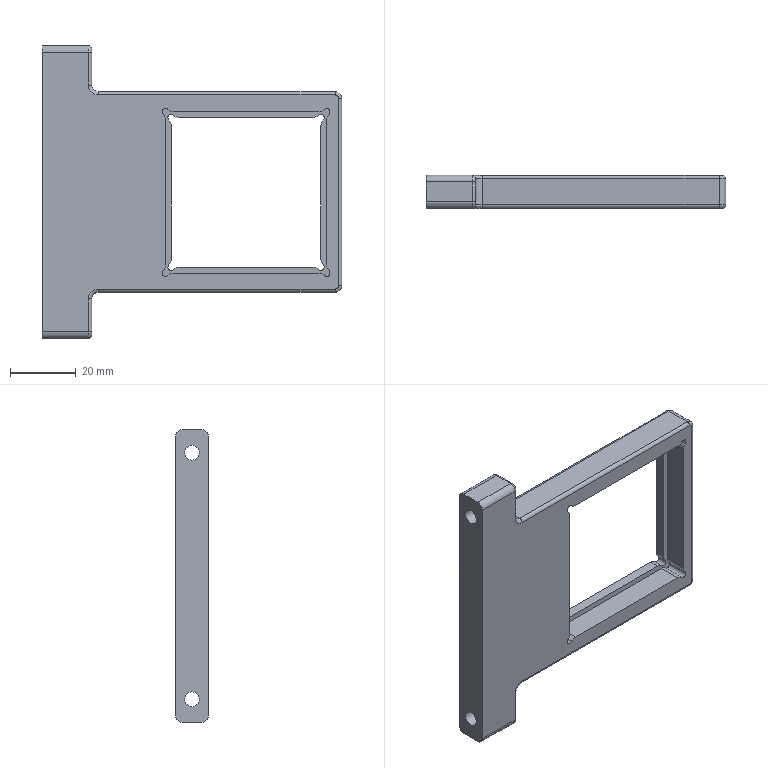NC program | NX | posted by the shop | part box 91 x 10 x 89 mm
Lines 39 to 1092 of 16928:
N2 T09 M06
(D10  D=10. R=0. H=09 ce=0.10 di=0.10)
G00 G90 G54 X33.301 Y3.249 M03 S8000
G43 H09 Z10.2
M08
Z1.5
G02 X33.301 Y3.249 Z1.006 I-2.966 J-3.384 F3000.
X33.301 Y3.249 Z.513 I-2.966 J-3.384
X33.301 Y3.249 Z.019 I-2.966 J-3.384
X33.301 Y3.249 Z-.474 I-2.966 J-3.384
X34.017 Y2.453 Z-.493 I-2.966 J-3.384
G01 X35.835 Y-.135
Y-19.535
X-2.965
Y19.265
X35.835
Y-2.121
G02 X35.417 Y-2.934 I-1. J0.0
G01 X29.254 Y-7.336
G03 X28.835 Y-8.149 I.581 J-.814
G01 Y-11.536
G02 X27.836 Y-12.535 I-1. J.001
G01 X5.034
G02 X4.035 Y-11.536 I.001 J1.
G01 Y11.266
G02 X5.034 Y12.265 I1. J-.001
G01 X27.836
G02 X28.835 Y11.266 I-.001 J-1.
G01 Y-1.878
G02 X28.107 Y-2.84 I-1. J0.0
G01 X22.354 Y-4.462
G03 X21.731 Y-4.98 I.272 J-.962
G02 X20.836 Y-5.535 I-.896 J.445
G01 X12.034
G02 X11.035 Y-4.536 I.001 J1.
G01 Y4.266
G02 X12.034 Y5.265 I1. J-.001
G01 X20.836
G02 X21.835 Y4.266 I-.001 J-1.
G01 X21.833 Y-1.135
G02 X21.033 Y-1.935 I-.8 J0.0
G01 X20.877 Y-1.919
X16.63 Y-1.074
G03 X16.34 Y-1.03 I-.631 J-3.173
G02 X15.535 Y-.135 I.095 J.895
X16.435 Y.765 I.9 J0.0
X17.335 Y-.135 I0.0 J-.9
X17.128 Y-.709 I-.9 J0.0
X16.721 Y-.988 I-.693 J.574
G03 X11.943 Y-7.626 I2.222 J-6.638
X12.305 Y-9.848 I7. J0.0
G01 Z.707
G00 Z3.
G01 X33.301 Y3.249 F6000.
G00 Z1.007
G02 X33.301 Y3.249 Z.514 I-2.966 J-3.384 F3000.
X33.301 Y3.249 Z.02 I-2.966 J-3.384
X33.301 Y3.249 Z-.473 I-2.966 J-3.384
X33.301 Y3.249 Z-.967 I-2.966 J-3.384
X34.017 Y2.453 Z-.986 I-2.966 J-3.384
G01 X35.835 Y-.135
Y-19.535
X-2.965
Y19.265
X35.835
Y-5.135
G02 X35.073 Y-6.106 I-1. J0.0
G01 X29.597 Y-7.448
G03 X28.835 Y-8.419 I.238 J-.971
G01 Y-11.536
G02 X27.836 Y-12.535 I-1. J.001
G01 X5.034
G02 X4.035 Y-11.536 I.001 J1.
G01 Y11.266
G02 X5.034 Y12.265 I1. J-.001
G01 X27.836
G02 X28.835 Y11.266 I-.001 J-1.
G01 Y-1.878
G02 X28.107 Y-2.84 I-1. J0.0
G01 X22.354 Y-4.462
G03 X21.731 Y-4.98 I.272 J-.962
G02 X20.837 Y-5.535 I-.896 J.445
G01 X12.034
G02 X11.035 Y-4.536 I.002 J1.
G01 Y4.267
G02 X12.034 Y5.265 I1. J-.002
G01 X20.837
G02 X21.835 Y4.267 I-.002 J-1.
G01 X21.833 Y-1.135
G02 X21.033 Y-1.935 I-.8 J0.0
G01 X20.877 Y-1.919
X16.63 Y-1.074
G03 X16.34 Y-1.03 I-.631 J-3.174
G02 X15.535 Y-.135 I.095 J.895
X16.435 Y.765 I.9 J0.0
X17.335 Y-.135 I0.0 J-.9
X17.128 Y-.709 I-.9 J0.0
X16.721 Y-.988 I-.693 J.574
G03 X11.943 Y-7.626 I2.222 J-6.638
X12.305 Y-9.848 I7. J0.0
G01 Z.214
G00 Z2.507
G01 X33.301 Y3.249 F6000.
G00 Z.514
G02 X33.301 Y3.249 Z.021 I-2.966 J-3.384 F3000.
X33.301 Y3.249 Z-.473 I-2.966 J-3.384
X33.301 Y3.249 Z-.966 I-2.966 J-3.384
X33.301 Y3.249 Z-1.46 I-2.966 J-3.384
X34.017 Y2.453 Z-1.479 I-2.966 J-3.384
G01 X35.835 Y-.135
Y-19.535
X-2.965
Y19.265
X35.835
Y-5.135
G02 X35.073 Y-6.106 I-1. J0.0
G01 X29.597 Y-7.448
G03 X28.835 Y-8.419 I.238 J-.971
G01 Y-11.535
G02 X27.836 Y-12.535 I-1. J0.0
G01 X5.035
G02 X4.035 Y-11.535 I0.0 J1.
G01 Y11.266
G02 X5.035 Y12.265 I1. J0.0
G01 X27.836
G02 X28.835 Y11.266 I0.0 J-1.
G01 Y-1.878
G02 X28.107 Y-2.84 I-1. J0.0
G01 X22.354 Y-4.462
G03 X21.731 Y-4.98 I.272 J-.962
G02 X20.836 Y-5.535 I-.896 J.445
G01 X12.034
G02 X11.035 Y-4.536 I.001 J1.
G01 Y4.266
G02 X12.034 Y5.265 I1. J-.001
G01 X20.836
G02 X21.835 Y4.266 I-.001 J-1.
G01 X21.833 Y-1.135
G02 X21.033 Y-1.935 I-.8 J0.0
G01 X20.877 Y-1.919
X16.631 Y-1.074
G03 X16.341 Y-1.03 I-.631 J-3.173
G02 X15.535 Y-.135 I.095 J.895
X16.435 Y.765 I.9 J0.0
X17.335 Y-.135 I0.0 J-.9
X17.128 Y-.709 I-.9 J0.0
X16.721 Y-.988 I-.693 J.574
G03 X11.943 Y-7.626 I2.222 J-6.638
X12.305 Y-9.848 I7. J0.0
G01 Z-.279
G00 Z2.014
G01 X33.301 Y3.249 F6000.
G00 Z.021
G02 X33.301 Y3.249 Z-.472 I-2.966 J-3.384 F3000.
X33.301 Y3.249 Z-.966 I-2.966 J-3.384
X33.301 Y3.249 Z-1.459 I-2.966 J-3.384
X33.301 Y3.249 Z-1.953 I-2.966 J-3.384
X34.017 Y2.453 Z-1.971 I-2.966 J-3.384
G01 X35.835 Y-.135
Y-19.535
X-2.965
Y19.265
X35.835
Y-5.135
G02 X35.073 Y-6.106 I-1. J0.0
G01 X29.597 Y-7.448
G03 X28.835 Y-8.419 I.238 J-.971
G01 Y-11.535
G02 X27.836 Y-12.535 I-1. J0.0
G01 X5.035
G02 X4.035 Y-11.535 I0.0 J1.
G01 Y11.266
G02 X5.035 Y12.265 I1. J0.0
G01 X27.836
G02 X28.835 Y11.266 I0.0 J-1.
G01 Y-1.878
G02 X28.107 Y-2.84 I-1. J0.0
G01 X22.354 Y-4.462
G03 X21.731 Y-4.98 I.272 J-.962
G02 X20.836 Y-5.535 I-.896 J.445
G01 X12.034
G02 X11.035 Y-4.536 I.001 J1.
G01 Y4.266
G02 X12.034 Y5.265 I1. J-.001
G01 X20.836
G02 X21.835 Y4.266 I-.001 J-1.
G01 X21.833 Y-1.135
G02 X21.033 Y-1.935 I-.8 J0.0
G01 X20.877 Y-1.919
X16.631 Y-1.074
G03 X16.341 Y-1.03 I-.631 J-3.173
G02 X15.535 Y-.135 I.095 J.895
X16.435 Y.765 I.9 J0.0
X17.335 Y-.135 I0.0 J-.9
X17.128 Y-.709 I-.9 J0.0
X16.721 Y-.988 I-.693 J.574
G03 X11.943 Y-7.626 I2.222 J-6.638
X12.305 Y-9.848 I7. J0.0
G01 Z-.771
G00 Z1.521
G01 X33.301 Y3.249 F6000.
G00 Z-.471
G02 X33.301 Y3.249 Z-.965 I-2.966 J-3.384 F3000.
X33.301 Y3.249 Z-1.458 I-2.966 J-3.384
X33.301 Y3.249 Z-1.952 I-2.966 J-3.384
X33.301 Y3.249 Z-2.446 I-2.966 J-3.384
X34.017 Y2.453 Z-2.464 I-2.966 J-3.384
G01 X35.835 Y-.135
Y-19.535
X-2.965
Y19.265
X35.835
Y-5.135
G02 X35.073 Y-6.106 I-1. J0.0
G01 X29.597 Y-7.448
G03 X28.835 Y-8.419 I.238 J-.971
G01 Y-11.535
G02 X27.836 Y-12.535 I-1. J0.0
G01 X5.035
G02 X4.035 Y-11.535 I0.0 J1.
G01 Y11.266
G02 X5.035 Y12.265 I1. J0.0
G01 X27.836
G02 X28.835 Y11.266 I0.0 J-1.
G01 Y-1.878
G02 X28.107 Y-2.84 I-1. J0.0
G01 X22.354 Y-4.462
G03 X21.731 Y-4.98 I.272 J-.962
G02 X20.836 Y-5.535 I-.896 J.445
G01 X12.034
G02 X11.035 Y-4.536 I.001 J1.
G01 Y4.266
G02 X12.034 Y5.265 I1. J-.001
G01 X20.836
G02 X21.835 Y4.266 I-.001 J-1.
G01 X21.833 Y-1.135
G02 X21.033 Y-1.935 I-.8 J0.0
G01 X20.877 Y-1.919
X16.631 Y-1.074
G03 X16.341 Y-1.03 I-.631 J-3.173
G02 X15.535 Y-.135 I.095 J.895
X16.435 Y.765 I.9 J0.0
X17.335 Y-.135 I0.0 J-.9
X17.128 Y-.709 I-.9 J0.0
X16.721 Y-.988 I-.693 J.574
G03 X11.943 Y-7.626 I2.222 J-6.638
X12.305 Y-9.848 I7. J0.0
G01 Z-1.264
G00 Z1.029
G01 X33.301 Y3.249 F6000.
G00 Z-.964
G02 X33.301 Y3.249 Z-1.458 I-2.966 J-3.384 F3000.
X33.301 Y3.249 Z-1.951 I-2.966 J-3.384
X33.301 Y3.249 Z-2.445 I-2.966 J-3.384
X33.301 Y3.249 Z-2.938 I-2.966 J-3.384
X34.017 Y2.453 Z-2.957 I-2.966 J-3.384
G01 X35.835 Y-.135
Y-19.535
X-2.965
Y19.265
X35.835
Y-5.135
G02 X35.073 Y-6.106 I-1. J0.0
G01 X29.597 Y-7.448
G03 X28.835 Y-8.419 I.238 J-.971
G01 Y-11.535
G02 X27.836 Y-12.535 I-1. J0.0
G01 X5.035
G02 X4.035 Y-11.535 I0.0 J1.
G01 Y11.266
G02 X5.035 Y12.265 I1. J0.0
G01 X27.836
G02 X28.835 Y11.266 I0.0 J-1.
G01 Y-1.878
G02 X28.107 Y-2.84 I-1. J0.0
G01 X22.354 Y-4.462
G03 X21.731 Y-4.98 I.272 J-.962
G02 X20.836 Y-5.535 I-.896 J.445
G01 X12.034
G02 X11.035 Y-4.536 I.001 J1.
G01 Y4.266
G02 X12.034 Y5.265 I1. J-.001
G01 X20.836
G02 X21.835 Y4.266 I-.001 J-1.
G01 X21.833 Y-1.135
G02 X21.033 Y-1.935 I-.8 J0.0
G01 X20.877 Y-1.919
X16.631 Y-1.074
G03 X16.341 Y-1.03 I-.631 J-3.173
G02 X15.535 Y-.135 I.095 J.895
X16.435 Y.765 I.9 J0.0
X17.335 Y-.135 I0.0 J-.9
X17.128 Y-.709 I-.9 J0.0
X16.721 Y-.988 I-.693 J.574
G03 X11.943 Y-7.626 I2.222 J-6.638
X12.305 Y-9.848 I7. J0.0
G01 Z-1.757
G00 Z.536
G01 X33.301 Y3.249 F6000.
G00 Z-1.457
G02 X33.301 Y3.249 Z-1.951 I-2.966 J-3.384 F3000.
X33.301 Y3.249 Z-2.444 I-2.966 J-3.384
X33.301 Y3.249 Z-2.938 I-2.966 J-3.384
X33.301 Y3.249 Z-3.431 I-2.966 J-3.384
X34.017 Y2.453 Z-3.45 I-2.966 J-3.384
G01 X35.835 Y-.135
Y-19.535
X-2.965
Y19.265
X35.835
Y-5.135
G02 X35.073 Y-6.106 I-1. J0.0
G01 X29.597 Y-7.448
G03 X28.835 Y-8.419 I.238 J-.971
G01 Y-11.535
G02 X27.836 Y-12.535 I-1. J0.0
G01 X5.035
G02 X4.035 Y-11.535 I0.0 J1.
G01 Y11.266
G02 X5.035 Y12.265 I1. J0.0
G01 X27.836
G02 X28.835 Y11.266 I0.0 J-1.
G01 Y-1.878
G02 X28.107 Y-2.84 I-1. J0.0
G01 X22.354 Y-4.462
G03 X21.731 Y-4.98 I.272 J-.962
G02 X20.836 Y-5.535 I-.896 J.445
G01 X12.034
G02 X11.035 Y-4.536 I.001 J1.
G01 Y4.266
G02 X12.034 Y5.265 I1. J-.001
G01 X20.836
G02 X21.835 Y4.266 I-.001 J-1.
G01 X21.833 Y-1.135
G02 X21.033 Y-1.935 I-.8 J0.0
G01 X20.877 Y-1.919
X16.631 Y-1.074
G03 X16.341 Y-1.03 I-.631 J-3.173
G02 X15.535 Y-.135 I.095 J.895
X16.435 Y.765 I.9 J0.0
X17.335 Y-.135 I0.0 J-.9
X17.128 Y-.709 I-.9 J0.0
X16.721 Y-.988 I-.693 J.574
G03 X11.943 Y-7.626 I2.222 J-6.638
X12.305 Y-9.848 I7. J0.0
G01 Z-2.25
G00 Z.043
G01 X33.301 Y3.249 F6000.
G00 Z-1.95
G02 X33.301 Y3.249 Z-2.444 I-2.966 J-3.384 F3000.
X33.301 Y3.249 Z-2.937 I-2.966 J-3.384
X33.301 Y3.249 Z-3.431 I-2.966 J-3.384
X33.301 Y3.249 Z-3.924 I-2.966 J-3.384
X34.017 Y2.453 Z-3.943 I-2.966 J-3.384
G01 X35.835 Y-.135
Y-19.535
X-2.965
Y19.265
X35.835
Y-5.135
G02 X35.073 Y-6.106 I-1. J0.0
G01 X29.597 Y-7.448
G03 X28.835 Y-8.419 I.238 J-.971
G01 Y-11.535
G02 X27.836 Y-12.535 I-1. J0.0
G01 X5.035
G02 X4.035 Y-11.535 I0.0 J1.
G01 Y11.266
G02 X5.035 Y12.265 I1. J0.0
G01 X27.836
G02 X28.835 Y11.266 I0.0 J-1.
G01 Y-1.878
G02 X28.107 Y-2.84 I-1. J0.0
G01 X22.354 Y-4.462
G03 X21.731 Y-4.98 I.272 J-.962
G02 X20.836 Y-5.535 I-.896 J.445
G01 X12.034
G02 X11.035 Y-4.536 I.001 J1.
G01 Y4.266
G02 X12.034 Y5.265 I1. J-.001
G01 X20.836
G02 X21.835 Y4.266 I-.001 J-1.
G01 X21.833 Y-1.135
G02 X21.033 Y-1.935 I-.8 J0.0
G01 X20.877 Y-1.919
X16.631 Y-1.074
G03 X16.341 Y-1.03 I-.631 J-3.173
G02 X15.535 Y-.135 I.095 J.895
X16.435 Y.765 I.9 J0.0
X17.335 Y-.135 I0.0 J-.9
X17.128 Y-.709 I-.9 J0.0
X16.721 Y-.988 I-.693 J.574
G03 X11.943 Y-7.626 I2.222 J-6.638
X12.305 Y-9.848 I7. J0.0
G01 Z-2.743
G00 Z-.45
G01 X33.301 Y3.249 F6000.
G00 Z-2.443
G02 X33.301 Y3.249 Z-2.936 I-2.966 J-3.384 F3000.
X33.301 Y3.249 Z-3.43 I-2.966 J-3.384
X33.301 Y3.249 Z-3.923 I-2.966 J-3.384
X33.301 Y3.249 Z-4.417 I-2.966 J-3.384
X34.017 Y2.453 Z-4.436 I-2.966 J-3.384
G01 X35.835 Y-.135
Y-19.535
X-2.965
Y19.265
X35.835
Y-5.135
G02 X35.073 Y-6.106 I-1. J0.0
G01 X29.597 Y-7.448
G03 X28.835 Y-8.419 I.238 J-.971
G01 Y-11.535
G02 X27.836 Y-12.535 I-1. J0.0
G01 X5.035
G02 X4.035 Y-11.535 I0.0 J1.
G01 Y11.266
G02 X5.035 Y12.265 I1. J0.0
G01 X27.836
G02 X28.835 Y11.266 I0.0 J-1.
G01 Y-1.878
G02 X28.107 Y-2.84 I-1. J0.0
G01 X22.354 Y-4.462
G03 X21.731 Y-4.98 I.272 J-.962
G02 X20.836 Y-5.535 I-.896 J.445
G01 X12.034
G02 X11.035 Y-4.536 I.001 J1.
G01 Y4.266
G02 X12.034 Y5.265 I1. J-.001
G01 X20.836
G02 X21.835 Y4.266 I-.001 J-1.
G01 X21.833 Y-1.135
G02 X21.033 Y-1.935 I-.8 J0.0
G01 X20.877 Y-1.919
X16.631 Y-1.074
G03 X16.341 Y-1.03 I-.631 J-3.173
G02 X15.535 Y-.135 I.095 J.895
X16.435 Y.765 I.9 J0.0
X17.335 Y-.135 I0.0 J-.9
X17.128 Y-.709 I-.9 J0.0
X16.721 Y-.988 I-.693 J.574
G03 X11.943 Y-7.626 I2.222 J-6.638
X12.305 Y-9.848 I7. J0.0
G01 Z-3.236
G00 Z-.943
G01 X33.301 Y3.249 F6000.
G00 Z-2.936
G02 X33.301 Y3.249 Z-3.429 I-2.966 J-3.384 F3000.
X33.301 Y3.249 Z-3.923 I-2.966 J-3.384
X33.301 Y3.249 Z-4.416 I-2.966 J-3.384
X33.301 Y3.249 Z-4.91 I-2.966 J-3.384
X34.017 Y2.453 Z-4.929 I-2.966 J-3.384
G01 X35.835 Y-.135
Y-19.535
X-2.965
Y19.265
X35.835
Y-5.135
G02 X35.073 Y-6.106 I-1. J0.0
G01 X29.597 Y-7.448
G03 X28.835 Y-8.419 I.238 J-.971
G01 Y-11.535
G02 X27.836 Y-12.535 I-1. J0.0
G01 X5.035
G02 X4.035 Y-11.535 I0.0 J1.
G01 Y11.266
G02 X5.035 Y12.265 I1. J0.0
G01 X27.836
G02 X28.835 Y11.266 I0.0 J-1.
G01 Y-1.878
G02 X28.107 Y-2.84 I-1. J0.0
G01 X22.354 Y-4.462
G03 X21.731 Y-4.98 I.272 J-.962
G02 X20.836 Y-5.535 I-.896 J.445
G01 X12.034
G02 X11.035 Y-4.536 I.001 J1.
G01 Y4.266
G02 X12.034 Y5.265 I1. J-.001
G01 X20.836
G02 X21.835 Y4.266 I-.001 J-1.
G01 X21.833 Y-1.135
G02 X21.033 Y-1.935 I-.8 J0.0
G01 X20.877 Y-1.919
X16.631 Y-1.074
G03 X16.341 Y-1.03 I-.631 J-3.173
G02 X15.535 Y-.135 I.095 J.895
X16.435 Y.765 I.9 J0.0
X17.335 Y-.135 I0.0 J-.9
X17.128 Y-.709 I-.9 J0.0
X16.721 Y-.988 I-.693 J.574
G03 X11.943 Y-7.626 I2.222 J-6.638
X12.305 Y-9.848 I7. J0.0
G01 Z-3.729
G00 Z-1.436
G01 X33.301 Y3.249 F6000.
G00 Z-3.429
G02 X33.301 Y3.249 Z-3.922 I-2.966 J-3.384 F3000.
X33.301 Y3.249 Z-4.416 I-2.966 J-3.384
X33.301 Y3.249 Z-4.909 I-2.966 J-3.384
X33.301 Y3.249 Z-5.403 I-2.966 J-3.384
X34.017 Y2.453 Z-5.421 I-2.966 J-3.384
G01 X35.835 Y-.135
Y-19.535
X-2.965
Y19.265
X35.835
Y-5.135
G02 X35.073 Y-6.106 I-1. J0.0
G01 X29.597 Y-7.448
G03 X28.835 Y-8.419 I.238 J-.971
G01 Y-11.535
G02 X27.836 Y-12.535 I-1. J0.0
G01 X5.035
G02 X4.035 Y-11.535 I0.0 J1.
G01 Y11.266
G02 X5.035 Y12.265 I1. J0.0
G01 X27.836
G02 X28.835 Y11.266 I0.0 J-1.
G01 Y-1.878
G02 X28.107 Y-2.84 I-1. J0.0
G01 X22.354 Y-4.462
G03 X21.731 Y-4.98 I.272 J-.962
G02 X20.836 Y-5.535 I-.896 J.445
G01 X12.034
G02 X11.035 Y-4.536 I.001 J1.
G01 Y4.266
G02 X12.034 Y5.265 I1. J-.001
G01 X20.836
G02 X21.835 Y4.266 I-.001 J-1.
G01 X21.833 Y-1.135
G02 X21.033 Y-1.935 I-.8 J0.0
G01 X20.877 Y-1.919
X16.631 Y-1.074
G03 X16.341 Y-1.03 I-.631 J-3.173
G02 X15.535 Y-.135 I.095 J.895
X16.435 Y.765 I.9 J0.0
X17.335 Y-.135 I0.0 J-.9
X17.128 Y-.709 I-.9 J0.0
X16.721 Y-.988 I-.693 J.574
G03 X11.943 Y-7.626 I2.222 J-6.638
X12.305 Y-9.848 I7. J0.0
G01 Z-4.221
G00 Z-1.929
G01 X33.301 Y3.249 F6000.
G00 Z-3.921
G02 X33.301 Y3.249 Z-4.415 I-2.966 J-3.384 F3000.
X33.301 Y3.249 Z-4.908 I-2.966 J-3.384
X33.301 Y3.249 Z-5.402 I-2.966 J-3.384
X33.301 Y3.249 Z-5.896 I-2.966 J-3.384
X34.017 Y2.453 Z-5.914 I-2.966 J-3.384
G01 X35.835 Y-.135
Y-19.535
X-2.965
Y19.265
X35.835
Y-5.135
G02 X35.073 Y-6.106 I-1. J0.0
G01 X29.597 Y-7.448
G03 X28.835 Y-8.419 I.238 J-.971
G01 Y-11.535
G02 X27.836 Y-12.535 I-1. J0.0
G01 X5.035
G02 X4.035 Y-11.535 I0.0 J1.
G01 Y11.266
G02 X5.035 Y12.265 I1. J0.0
G01 X27.836
G02 X28.835 Y11.266 I0.0 J-1.
G01 Y-1.878
G02 X28.107 Y-2.84 I-1. J0.0
G01 X22.354 Y-4.462
G03 X21.731 Y-4.98 I.272 J-.962
G02 X20.836 Y-5.535 I-.896 J.445
G01 X12.034
G02 X11.035 Y-4.536 I.001 J1.
G01 Y4.266
G02 X12.034 Y5.265 I1. J-.001
G01 X20.836
G02 X21.835 Y4.266 I-.001 J-1.
G01 X21.833 Y-1.135
G02 X21.033 Y-1.935 I-.8 J0.0
G01 X20.877 Y-1.919
X16.631 Y-1.074
G03 X16.341 Y-1.03 I-.631 J-3.173
G02 X15.535 Y-.135 I.095 J.895
X16.435 Y.765 I.9 J0.0
X17.335 Y-.135 I0.0 J-.9
X17.128 Y-.709 I-.9 J0.0
X16.721 Y-.988 I-.693 J.574
G03 X11.943 Y-7.626 I2.222 J-6.638
X12.305 Y-9.848 I7. J0.0
G01 Z-4.714
G00 Z-2.421
G01 X33.301 Y3.249 F6000.
G00 Z-4.414
G02 X33.301 Y3.249 Z-4.908 I-2.966 J-3.384 F3000.
X33.301 Y3.249 Z-5.401 I-2.966 J-3.384
X33.301 Y3.249 Z-5.895 I-2.966 J-3.384
X33.301 Y3.249 Z-6.388 I-2.966 J-3.384
X34.017 Y2.453 Z-6.407 I-2.966 J-3.384
G01 X35.835 Y-.135
Y-19.535
X-2.965
Y19.265
X35.835
Y-5.135
G02 X35.073 Y-6.106 I-1. J0.0
G01 X29.597 Y-7.448
G03 X28.835 Y-8.419 I.238 J-.971
G01 Y-11.535
G02 X27.836 Y-12.535 I-1. J0.0
G01 X5.035
G02 X4.035 Y-11.535 I0.0 J1.
G01 Y11.266
G02 X5.035 Y12.265 I1. J0.0
G01 X27.836
G02 X28.835 Y11.266 I0.0 J-1.
G01 Y-1.878
G02 X28.107 Y-2.84 I-1. J0.0
G01 X22.354 Y-4.462
G03 X21.731 Y-4.98 I.272 J-.962
G02 X20.836 Y-5.535 I-.896 J.445
G01 X12.034
G02 X11.035 Y-4.536 I.001 J1.
G01 Y4.266
G02 X12.034 Y5.265 I1. J-.001
G01 X20.836
G02 X21.835 Y4.266 I-.001 J-1.
G01 X21.833 Y-1.135
G02 X21.033 Y-1.935 I-.8 J0.0
G01 X20.877 Y-1.919
X16.631 Y-1.074
G03 X16.341 Y-1.03 I-.631 J-3.173
G02 X15.535 Y-.135 I.095 J.895
X16.435 Y.765 I.9 J0.0
X17.335 Y-.135 I0.0 J-.9
X17.128 Y-.709 I-.9 J0.0
X16.721 Y-.988 I-.693 J.574
G03 X11.943 Y-7.626 I2.222 J-6.638
X12.305 Y-9.848 I7. J0.0
G01 Z-5.207
G00 Z-2.914
G01 X33.301 Y3.249 F6000.
G00 Z-4.907
G02 X33.301 Y3.249 Z-5.401 I-2.966 J-3.384 F3000.
X33.301 Y3.249 Z-5.894 I-2.966 J-3.384
X33.301 Y3.249 Z-6.388 I-2.966 J-3.384
X33.301 Y3.249 Z-6.881 I-2.966 J-3.384
X34.017 Y2.453 Z-6.9 I-2.966 J-3.384
G01 X35.835 Y-.135
Y-19.535
X-2.965
Y19.265
X35.835
Y-5.135
G02 X35.073 Y-6.106 I-1. J0.0
G01 X29.597 Y-7.448
G03 X28.835 Y-8.419 I.238 J-.971
G01 Y-11.535
G02 X27.836 Y-12.535 I-1. J0.0
G01 X5.035
G02 X4.035 Y-11.535 I0.0 J1.
G01 Y11.266
G02 X5.035 Y12.265 I1. J0.0
G01 X27.836
G02 X28.835 Y11.266 I0.0 J-1.
G01 Y-1.878
G02 X28.107 Y-2.84 I-1. J0.0
G01 X22.354 Y-4.462
G03 X21.731 Y-4.98 I.272 J-.962
G02 X20.836 Y-5.535 I-.896 J.445
G01 X12.034
G02 X11.035 Y-4.536 I.001 J1.
G01 Y4.266
G02 X12.034 Y5.265 I1. J-.001
G01 X20.836
G02 X21.835 Y4.266 I-.001 J-1.
G01 X21.833 Y-1.135
G02 X21.033 Y-1.935 I-.8 J0.0
G01 X20.877 Y-1.919
X16.631 Y-1.074
G03 X16.341 Y-1.03 I-.631 J-3.173
G02 X15.535 Y-.135 I.095 J.895
X16.435 Y.765 I.9 J0.0
X17.335 Y-.135 I0.0 J-.9
X17.128 Y-.709 I-.9 J0.0
X16.721 Y-.988 I-.693 J.574
G03 X11.943 Y-7.626 I2.222 J-6.638
X12.305 Y-9.848 I7. J0.0
G01 Z-5.7
G00 Z-3.407
G01 X32.353 Y2.325 F6000.
G00 Z-5.4
G02 X32.353 Y2.325 Z-5.894 I-3.768 J-2.46 F3000.
X32.353 Y2.325 Z-6.387 I-3.768 J-2.46
X32.353 Y2.325 Z-6.881 I-3.768 J-2.46
X32.267 Y2.453 Z-7.371 I-3.768 J-2.46
G01 X34.085 Y-.135
Y-17.785
X-1.215
Y17.515
X34.085
Y-5.135
G02 X33.323 Y-6.106 I-1. J0.0
G01 X27.847 Y-7.448
G03 X27.085 Y-8.419 I.238 J-.971
G01 Y-9.785
G02 X26.086 Y-10.785 I-1. J0.0
G01 X6.785
G02 X5.785 Y-9.785 I0.0 J1.
G01 Y9.516
G02 X6.785 Y10.515 I1. J0.0
G01 X26.086
G02 X27.085 Y9.516 I0.0 J-1.
G01 Y-1.695
G02 X26.147 Y-2.692 I-1. J0.0
G01 X20.587 Y-3.033
G03 X19.867 Y-3.408 I.062 J-.998
G02 X19.086 Y-3.785 I-.782 J.623
G01 X13.784
G02 X12.785 Y-2.786 I.001 J1.
G01 Y2.516
G02 X13.784 Y3.515 I1. J-.001
G01 X19.086
G02 X20.085 Y2.516 I-.001 J-1.
G01 Y-2.786
G02 X20.045 Y-3.067 I-1. J.001
X19.792 Y-3.492 I-.959 J.282
G03 X17.74 Y-8.443 I4.948 J-4.951
X19.789 Y-13.392 I7. J0.0
G01 Z-6.171
G00 Z-3.9
G01 X32.353 Y2.325 F6000.
G00 Z-5.871
G02 X32.353 Y2.325 Z-6.365 I-3.768 J-2.46 F3000.
X32.353 Y2.325 Z-6.858 I-3.768 J-2.46
X32.353 Y2.325 Z-7.352 I-3.768 J-2.46
X32.267 Y2.453 Z-7.843 I-3.768 J-2.46
G01 X34.085 Y-.135
Y-17.785
X-1.215
Y17.515
X34.085
Y-5.135
G02 X33.323 Y-6.106 I-1. J0.0
G01 X27.847 Y-7.448
G03 X27.085 Y-8.419 I.238 J-.971
G01 Y-9.785
G02 X26.086 Y-10.785 I-1. J0.0
G01 X6.785
G02 X5.785 Y-9.785 I0.0 J1.
G01 Y9.516
G02 X6.785 Y10.515 I1. J0.0
G01 X26.086
G02 X27.085 Y9.516 I0.0 J-1.
G01 Y-1.695
G02 X26.147 Y-2.692 I-1. J0.0
G01 X20.587 Y-3.033
G03 X19.867 Y-3.408 I.062 J-.998
G02 X19.086 Y-3.785 I-.782 J.623
G01 X13.784
G02 X12.785 Y-2.786 I.001 J1.
G01 Y2.516
G02 X13.784 Y3.515 I1. J-.001
G01 X19.086
G02 X20.085 Y2.516 I-.001 J-1.
G01 Y-2.786
G02 X20.045 Y-3.067 I-1. J.001
X19.792 Y-3.492 I-.959 J.282
G03 X17.74 Y-8.443 I4.948 J-4.951
X19.789 Y-13.392 I7. J0.0
G01 Z-6.643
G00 Z-4.371
G01 X32.353 Y2.325 F6000.
G00 Z-6.343
G02 X32.353 Y2.325 Z-6.836 I-3.768 J-2.46 F3000.
X32.353 Y2.325 Z-7.33 I-3.768 J-2.46
X32.353 Y2.325 Z-7.823 I-3.768 J-2.46
X32.267 Y2.453 Z-8.314 I-3.768 J-2.46
G01 X34.085 Y-.135
Y-17.785
X-1.215
Y17.515
X34.085
Y-5.135
G02 X33.323 Y-6.106 I-1. J0.0
G01 X27.847 Y-7.448
G03 X27.085 Y-8.419 I.238 J-.971
G01 Y-9.785
G02 X26.086 Y-10.785 I-1. J0.0
G01 X6.785
G02 X5.785 Y-9.785 I0.0 J1.
G01 Y9.516
G02 X6.785 Y10.515 I1. J0.0
G01 X26.086
G02 X27.085 Y9.516 I0.0 J-1.
G01 Y-1.695
G02 X26.147 Y-2.692 I-1. J0.0
G01 X20.587 Y-3.033
G03 X19.867 Y-3.408 I.062 J-.998
G02 X19.086 Y-3.785 I-.782 J.623
G01 X13.784
G02 X12.785 Y-2.786 I.001 J1.
G01 Y2.516
G02 X13.784 Y3.515 I1. J-.001
G01 X19.086
G02 X20.085 Y2.516 I-.001 J-1.
G01 Y-2.786
G02 X20.045 Y-3.067 I-1. J.001
X19.792 Y-3.492 I-.959 J.282
G03 X17.74 Y-8.443 I4.948 J-4.951
X19.789 Y-13.392 I7. J0.0
G01 Z-7.114
G00 Z-4.843
G01 X32.353 Y2.325 F6000.
G00 Z-6.814
G02 X32.353 Y2.325 Z-7.308 I-3.768 J-2.46 F3000.
X32.353 Y2.325 Z-7.801 I-3.768 J-2.46
X32.353 Y2.325 Z-8.295 I-3.768 J-2.46
X32.267 Y2.453 Z-8.786 I-3.768 J-2.46
G01 X34.085 Y-.135
Y-17.785
X-1.215
Y17.515
X34.085
Y-5.135
G02 X33.323 Y-6.106 I-1. J0.0
G01 X27.847 Y-7.448
G03 X27.085 Y-8.419 I.238 J-.971
G01 Y-9.785
G02 X26.086 Y-10.785 I-1. J0.0
G01 X6.785
G02 X5.785 Y-9.785 I0.0 J1.
G01 Y9.516
G02 X6.785 Y10.515 I1. J0.0
G01 X26.086
G02 X27.085 Y9.516 I0.0 J-1.
G01 Y-1.695
G02 X26.147 Y-2.692 I-1. J0.0
G01 X20.587 Y-3.033
G03 X19.867 Y-3.408 I.062 J-.998
G02 X19.086 Y-3.785 I-.782 J.623
G01 X13.784
G02 X12.785 Y-2.786 I.001 J1.
G01 Y2.516
G02 X13.784 Y3.515 I1. J-.001
G01 X19.086
G02 X20.085 Y2.516 I-.001 J-1.
G01 Y-2.786
G02 X20.045 Y-3.067 I-1. J.001
X19.792 Y-3.492 I-.959 J.282
G03 X17.74 Y-8.443 I4.948 J-4.951
X19.789 Y-13.392 I7. J0.0
G01 Z-7.586
G00 Z-5.314
G01 X32.353 Y2.325 F6000.
G00 Z-7.286
G02 X32.353 Y2.325 Z-7.779 I-3.768 J-2.46 F3000.
X32.353 Y2.325 Z-8.273 I-3.768 J-2.46
X32.353 Y2.325 Z-8.766 I-3.768 J-2.46
X32.267 Y2.453 Z-9.257 I-3.768 J-2.46
G01 X34.085 Y-.135
Y-17.785
X-1.215
Y17.515
X34.085
Y-5.135
G02 X33.323 Y-6.106 I-1. J0.0
G01 X27.847 Y-7.448
G03 X27.085 Y-8.419 I.238 J-.971
G01 Y-9.785
G02 X26.086 Y-10.785 I-1. J0.0
G01 X6.785
G02 X5.785 Y-9.785 I0.0 J1.
G01 Y9.516
G02 X6.785 Y10.515 I1. J0.0
G01 X26.086
G02 X27.085 Y9.516 I0.0 J-1.
G01 Y-1.695
G02 X26.147 Y-2.692 I-1. J0.0
G01 X20.587 Y-3.033
G03 X19.867 Y-3.408 I.062 J-.998
G02 X19.086 Y-3.785 I-.782 J.623
G01 X13.784
G02 X12.785 Y-2.786 I.001 J1.
G01 Y2.516
G02 X13.784 Y3.515 I1. J-.001
G01 X19.086
G02 X20.085 Y2.516 I-.001 J-1.
G01 Y-2.786
G02 X20.045 Y-3.067 I-1. J.001
X19.792 Y-3.492 I-.959 J.282
G03 X17.74 Y-8.443 I4.948 J-4.951
X19.789 Y-13.392 I7. J0.0
G01 Z-8.057
G00 Z-5.786
G01 X32.353 Y2.325 F6000.
G00 Z-7.757
G02 X32.353 Y2.325 Z-8.251 I-3.768 J-2.46 F3000.
X32.353 Y2.325 Z-8.744 I-3.768 J-2.46
X32.353 Y2.325 Z-9.238 I-3.768 J-2.46
X32.267 Y2.453 Z-9.729 I-3.768 J-2.46
G01 X34.085 Y-.135
Y-17.785
X-1.215
Y17.515
X34.085
Y-5.135
G02 X33.323 Y-6.106 I-1. J0.0
G01 X27.847 Y-7.448
G03 X27.085 Y-8.419 I.238 J-.971
G01 Y-9.785
G02 X26.086 Y-10.785 I-1. J0.0
G01 X6.785
G02 X5.785 Y-9.785 I0.0 J1.
G01 Y9.516
G02 X6.785 Y10.515 I1. J0.0
G01 X26.086
G02 X27.085 Y9.516 I0.0 J-1.
G01 Y-1.695
G02 X26.147 Y-2.692 I-1. J0.0
G01 X20.587 Y-3.033
G03 X19.867 Y-3.408 I.062 J-.998
G02 X19.086 Y-3.785 I-.782 J.623
G01 X13.784
G02 X12.785 Y-2.786 I.001 J1.
G01 Y2.516
G02 X13.784 Y3.515 I1. J-.001
G01 X19.086
G02 X20.085 Y2.516 I-.001 J-1.
G01 Y-2.786
G02 X20.045 Y-3.067 I-1. J.001
X19.792 Y-3.492 I-.959 J.282
G03 X17.74 Y-8.443 I4.948 J-4.951
X19.789 Y-13.392 I7. J0.0
G01 Z-8.529
G00 Z-6.257
G01 X32.353 Y2.325 F6000.
G00 Z-8.229
G02 X32.353 Y2.325 Z-8.722 I-3.768 J-2.46 F3000.
X32.353 Y2.325 Z-9.216 I-3.768 J-2.46
X32.353 Y2.325 Z-9.709 I-3.768 J-2.46
X32.267 Y2.453 Z-10.2 I-3.768 J-2.46
G01 X34.085 Y-.135
Y-17.785
X-1.215
Y17.515
X34.085
Y-5.135
G02 X33.323 Y-6.106 I-1. J0.0
G01 X27.847 Y-7.448
G03 X27.085 Y-8.419 I.238 J-.971
G01 Y-9.785
G02 X26.086 Y-10.785 I-1. J0.0
G01 X6.785
G02 X5.785 Y-9.785 I0.0 J1.
G01 Y9.516
G02 X6.785 Y10.515 I1. J0.0
G01 X26.086
G02 X27.085 Y9.516 I0.0 J-1.
G01 Y-1.695
G02 X26.147 Y-2.692 I-1. J0.0
G01 X20.587 Y-3.033
G03 X19.867 Y-3.408 I.062 J-.998
G02 X19.086 Y-3.785 I-.782 J.623
G01 X13.784
G02 X12.785 Y-2.786 I.001 J1.
G01 Y2.516
G02 X13.784 Y3.515 I1. J-.001
G01 X19.086
G02 X20.085 Y2.516 I-.001 J-1.
G01 Y-2.786
G02 X20.045 Y-3.067 I-1. J.001
X19.792 Y-3.492 I-.959 J.282
G03 X17.74 Y-8.443 I4.948 J-4.951
X19.789 Y-13.392 I7. J0.0
G01 Z-9.
G00 Z10.2
G00 G90 X15.685 Y-57. M03 S8000
Z10.2
Z.719
G01 Z-.481 F4000.
Y-52.5
G03 X8.685 Y-45.5 I-7. J0.0
G01 X-24.663
G02 X-27.243 Y-48.928 I-7.362 J2.856
X-29.28 Y-50. I-4.217 J5.542
G01 X-47.584
G02 X-52. Y-43.826 I2.108 J6.174
G01 Y-43.798
Y43.798
Y43.826
G02 X-47.584 Y50. I6.525 J0.0
G01 X-29.371
G02 X-24.655 Y45.5 I-2.26 J-7.089
G01 X48.
G02 X48.5 Y45. I0.0 J-.5
G01 Y37.668
G02 X47.5 Y36.668 I-1. J0.0
G01 X47.333 Y36.682
X42.276 Y37.537
X42.11 Y37.551
G03 X41.327 Y37.173 I0.0 J-1.
G02 X40.702 Y36.87 I-.627 J.497
G01 X-23.332
G02 X-24.131 Y37.67 I.002 J.801
G01 X-24.13 Y37.702
G02 X-23.332 Y38.5 I.8 J-.002
G01 X40.702
G02 X41.338 Y38.184 I-.002 J-.801
G03 X42.133 Y37.789 I.796 J.606
G01 X42.3 Y37.803
X47.333 Y38.654
X47.5 Y38.668
G02 X48.5 Y37.668 I0.0 J-1.
G01 Y35.212
G02 X51.87 Y28.5 I-5. J-6.712
G01 Y-28.5
G02 X48.5 Y-35.212 I-8.37 J0.0
G01 Y-45.
G02 X48. Y-45.5 I-.5 J0.0
G01 X3.685
G02 X2.714 Y-44.738 I0.0 J1.
G01 X1.372 Y-39.262
G03 X.401 Y-38.5 I-.971 J-.238
G01 X-23.332
G02 X-24.13 Y-37.702 I.002 J.8
G01 Y-37.668
G02 X-23.332 Y-36.87 I.8 J-.002
G01 X40.21
G03 X40.913 Y-36.425 I-.001 J.779
G01 X41.082 Y-36.07
X41.122 Y-35.89
G03 X40.702 Y-35.47 I-.42 J0.0
G01 X-25.53
Y-42.5
X-25.529 Y-42.644
G02 X-28.091 Y-47.814 I-6.496 J0.0
X-31.46 Y-48.95 I-3.37 J4.428
G01 X-45.5
G02 X-50.6 Y-43.826 I.024 J5.124
G01 Y-43.801
Y43.801
Y43.826
G02 X-45.5 Y48.95 I5.125 J0.0
G01 X-31.5
G02 X-25.738 Y44.239 I-.131 J-6.039
X-25.53 Y42.5 I-8.476 J-1.894
G01 Y35.47
X43.5
G02 X50.47 Y28.5 I0.0 J-6.97
G01 Y-28.5
G02 X43.5 Y-35.47 I-6.97 J0.0
G01 X40.702
G03 X40.282 Y-35.89 I0.0 J-.42